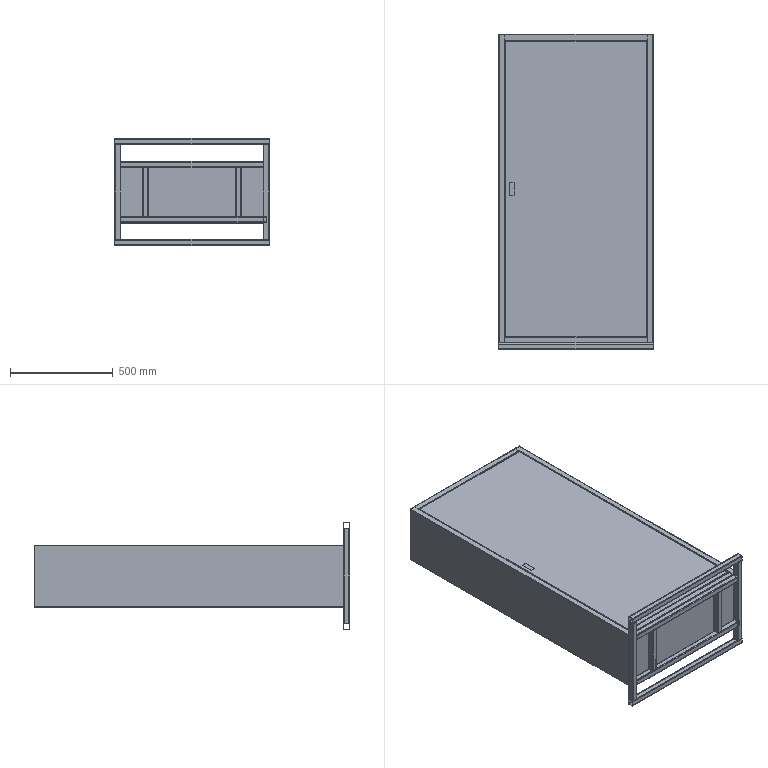Part | SolidWorks | features ICE 27, MoveFace 8, DelFace 7, FlatPattern 5, FlattenBends 5, ProcessBends 5, SheetMetal 5, CombineBodies 4, 3DProfileFeature 2, Extrusion 1, Fillet 1, LibraryFeature 1, Rip 1, Shell 1, Split 1, WeldMemberFeat 1, WeldmentFeature 1 | 14 solids | 452 faces | box 750 x 1530 x 520 mm | volume 6723347 mm3 | plane 322 | cylinder 114 | spline 16 | commonest cylinder face diameters 4 x32 8 x32 3.6 x22 0.6 x20 5.2 x8